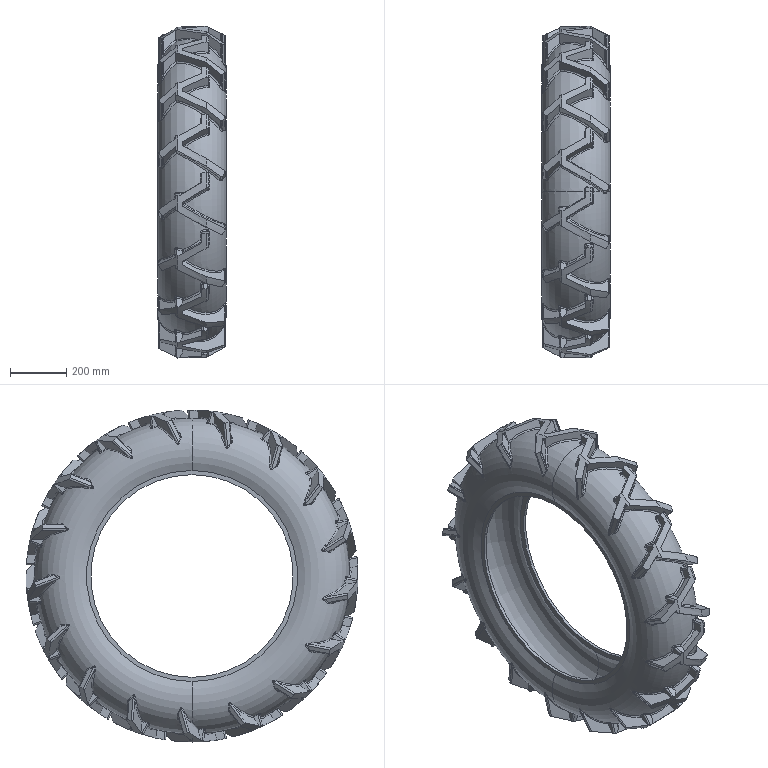Part | SolidWorks | 1 solid | 985 faces | box 244.595 x 1180 x 1180 mm | volume 23262229 mm3 | spline 306 | plane 276 | cylinder 226 | torus 106 | cone 54 | sphere 17 | commonest cylinder face diameters 10 x204 1180 x18 720 x4